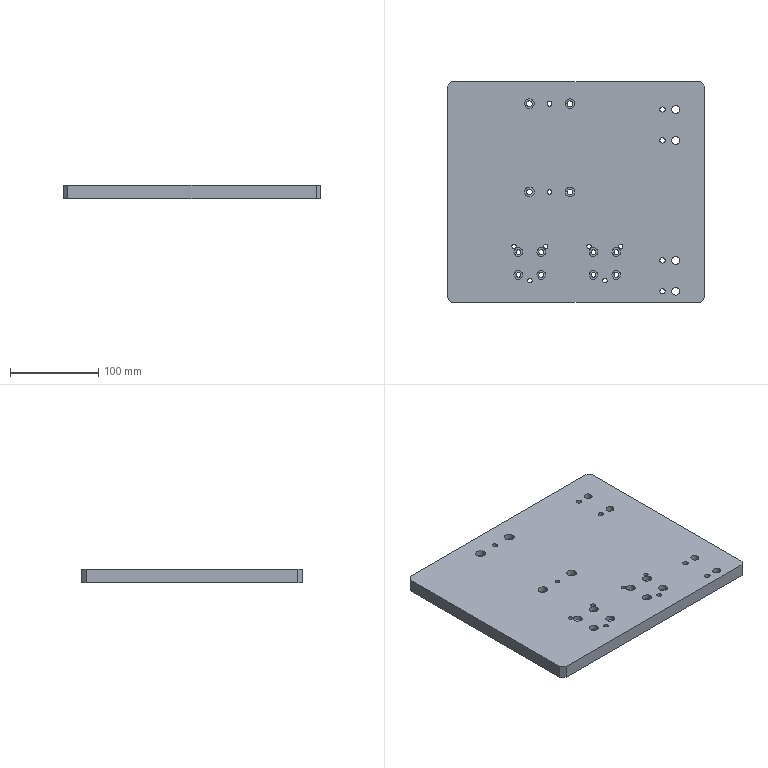CAM job | NX | 3-axis milling, drilling | part box 292 x 250 x 15 mm | stock box 298 x 256 x 16 mm
Tools:
number,name,description,diameter,corner_radius,flute_length,length,flutes
11,D10JING,Milling Tool-5 Parameters,10.0,0.0,50.0,75.0,2
7,D6A45,Milling Tool-5 Parameters,6.0,0.0,3.0,3.0,2
12,5.5ZT,Drilling Tool,5.5,0.0,35.0,50.0,2
16,6.6ZT,Drilling Tool,6.6,0.0,35.0,50.0,2
19,9.0ZT,Drilling Tool,9.0,0.0,35.0,50.0,2
14,4.8ZT,Drilling Tool,4.8,0.0,35.0,50.0,2
15,5.0JD,Milling Tool-5 Parameters,5.0,0.0,30.0,30.0,4
18,5.8ZT,Drilling Tool,5.8,0.0,35.0,50.0,2
20,6.0JD,Milling Tool-5 Parameters,6.0,0.0,30.0,30.0,4
10,D10,Milling Tool-5 Parameters,10.0,0.0,50.0,75.0,2
3,D3,Milling Tool-5 Parameters,3.0,0.0,50.0,75.0,2
6,D6,Milling Tool-5 Parameters,6.0,0.0,50.0,75.0,2
Operations:
program,operation,operation_type,tool,method,geometry_group,spindle_rpm,surface_speed,feed_per_tooth,feed_cut,feed_plunge,cut_length_mm,path_length_mm,cut_time_min,machine_time_min
1-295-253-15毛胚-AB胶,FLOOR_WALL,VolumeBased25DMillingOperation,D10JING,METHOD,A,6500.0,1286.0,0.0962,1250.0,100.0,13507.996,13561.996,10.806,10.812
1-295-253-15毛胚-AB胶,DRILLING_COPY_1,Operation,D6A45,METHOD,A,3000.0,56.0,0.0333,200.0,0.0,108.0,1155.237,0.54,0.6447
1-295-253-15毛胚-AB胶,DRILLING_COPY_1_COPY_COPY_1_COPY_1,Operation,5.5ZT,METHOD,A,2000.0,18.0,0.03,120.0,0.0,161.219,619.549,1.343,1.389
1-295-253-15毛胚-AB胶,DRILLING_COPY_1_COPY_COPY_1_COPY_1_COPY,Operation,6.6ZT,METHOD,A,2000.0,18.0,0.03,120.0,0.0,81.931,543.066,0.6828,0.7289
1-295-253-15毛胚-AB胶,DRILLING_COPY_1_COPY_COPY_1_COPY_1_COPY_1,Operation,9.0ZT,METHOD,A,2000.0,18.0,0.03,120.0,0.0,84.816,444.89,0.7068,0.7428
1-295-253-15毛胚-AB胶,DRILLING_COPY_1_COPY_COPY_1,Operation,4.8ZT,METHOD,A,2000.0,18.0,0.03,120.0,0.0,167.536,804.629,1.396,1.46
1-295-253-15毛胚-AB胶,DRILLING_COPY_1_COPY_COPY_1_COPY,Operation,5.0JD,METHOD,A,1000.0,9.0,0.01,40.0,0.0,129.5,625.011,3.237,3.287
1-295-253-15毛胚-AB胶,DRILLING_COPY_1_COPY_COPY_1_1,Operation,5.8ZT,METHOD,A,2000.0,18.0,0.03,120.0,0.0,84.97,445.199,0.7081,0.7441
1-295-253-15毛胚-AB胶,DRILLING_COPY_1_COPY_COPY_1_COPY_2,Operation,6.0JD,METHOD,A,1000.0,9.0,0.01,40.0,0.0,74.0,594.119,1.85,1.902
1-295-253-15毛胚-AB胶,ZLEVEL_PROFILE,ZLevelMilling,D10,METHOD,A,7000.0,219.0,0.2143,3000.0,1000.0,16668.547,16739.947,5.588,5.595
1-295-253-15毛胚-AB胶,HOLE_MILLING,CylinderMilling,D6,METHOD,A,7000.0,131.0,0.1071,1500.0,100.0,2299.767,3558.922,1.533,1.659
1-295-253-15毛胚-AB胶,ZLEVEL_PROFILE_COPY,ZLevelMilling,D3,METHOD,A,7000.0,65.0,0.0857,1200.0,1000.0,498.316,570.316,0.4208,0.428
1-295-253-15毛胚-AB胶,ZLEVEL_PROFILE_COPY_1_COPY_COPY_COPY_COPY_2_COPY,ZLevelMilling,D6A45,METHOD,A,7000.0,131.0,0.0714,1000.0,1000.0,1720.899,6310.221,1.721,2.18
1-295-253-15毛胚-AB胶,刀补4,ZLevelMilling,D3,METHOD,A,7000.0,87.0,0.0607,850.0,1000.0,128.034,203.634,0.1505,0.158
1-295-253-15毛胚-AB胶,ZLEVEL_PROFILE_COPY_1,ZLevelMilling,D10JING,METHOD,A,7000.0,219.0,0.0714,1000.0,1000.0,3353.271,3440.021,3.353,3.362